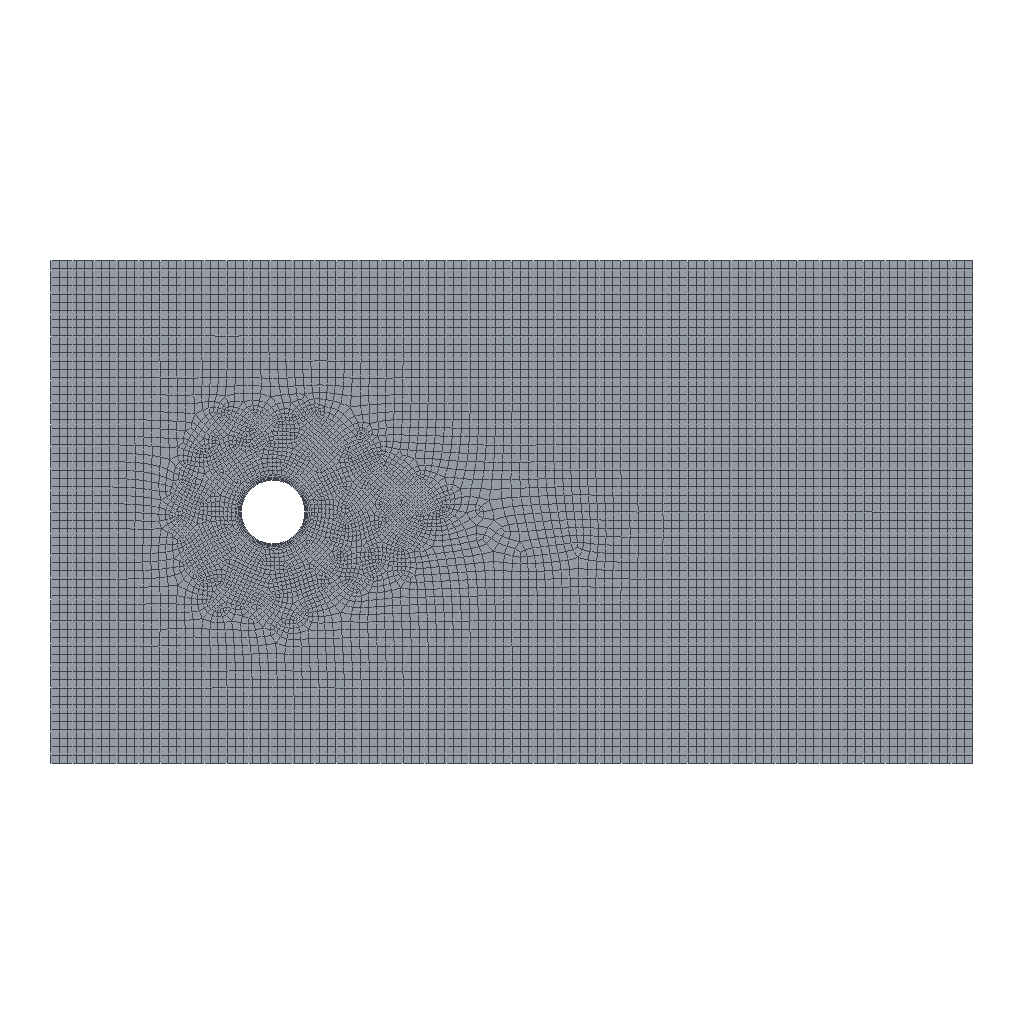Simulation study | ansys fluent
Set-up summary:
category,name,step,type,value,unit,region
solver,ansys_fluent,,Fluent 26.1.0
units,SI m-kg-s (Fluent internal),,stated,boundary values in the units shown in brackets; results in listed units
analysis,deck-1.cas,,"cfd unsteady, 1st-order implicit","dimension=2D; solver=2d, dp, pbns, LES, transient (2d, double precision, pressure-based, large eddy simulation, transient); source_case=2.cas"
model,Space,deck-1.cas,,2D
model,Time,deck-1.cas,,"Unsteady, 1st-Order Implicit"
model,Viscous,deck-1.cas,,Large Eddy Simulation
model,Sub-Grid Scale Model,deck-1.cas,,Smagorinsky-Lilly
model,Heat Transfer,deck-1.cas,,Disabled
model,Acoustics,deck-1.cas,,Ffowcs-Williams and Hawkings
model,Multiphase,deck-1.cas,,Disabled
analysis,deck-2.cas,,"cfd unsteady, 1st-order implicit","dimension=2D; solver=2d, dp, pbns, LES, transient (2d, double precision, pressure-based, large eddy simulation, transient); source_case=4.cas"
model,Space,deck-2.cas,,2D
model,Time,deck-2.cas,,"Unsteady, 1st-Order Implicit"
model,Viscous,deck-2.cas,,Large Eddy Simulation
model,Sub-Grid Scale Model,deck-2.cas,,Smagorinsky-Lilly
model,Heat Transfer,deck-2.cas,,Disabled
model,Multiphase,deck-2.cas,,Disabled
analysis,deck-3.cas,,"cfd unsteady, 1st-order implicit","dimension=2D; solver=2d, dp, pbns, LES, transient (2d, double precision, pressure-based, large eddy simulation, transient); source_case=5.cas.h5"
model,Space,deck-3.cas,,2D
model,Time,deck-3.cas,,"Unsteady, 1st-Order Implicit"
model,Viscous,deck-3.cas,,Large Eddy Simulation
model,Sub-Grid Scale Model,deck-3.cas,,Smagorinsky-Lilly
model,Heat Transfer,deck-3.cas,,Disabled
model,Multiphase,deck-3.cas,,Disabled
analysis,deck-4.cas,,"cfd unsteady, 1st-order implicit","dimension=2D; solver=2d, dp, pbns, LES, transient (2d, double precision, pressure-based, large eddy simulation, transient); source_case=.cas.h5"
model,Space,deck-4.cas,,2D
model,Time,deck-4.cas,,"Unsteady, 1st-Order Implicit"
model,Viscous,deck-4.cas,,Large Eddy Simulation
model,Sub-Grid Scale Model,deck-4.cas,,Smagorinsky-Lilly
model,Heat Transfer,deck-4.cas,,Disabled
model,Acoustics,deck-4.cas,,Ffowcs-Williams and Hawkings
model,Multiphase,deck-4.cas,,Disabled
mesh,deck-1.cas,,nodes,9109
mesh,deck-1.cas,,elements,8909
mesh,deck-1.cas,,faces,18018
mesh,deck-1.cas,,note,elements = cells; counts from the case file zone headers
mesh,deck-2.cas,,nodes,9109
mesh,deck-2.cas,,elements,8909
mesh,deck-2.cas,,faces,18018
mesh,deck-2.cas,,note,elements = cells; counts from the case file zone headers
mesh,deck-3.cas,,nodes,9109
mesh,deck-3.cas,,elements,8909
mesh,deck-3.cas,,faces,18018
mesh,deck-3.cas,,note,elements = cells; counts from the case file zone headers
mesh,deck-4.cas,,nodes,9109
mesh,deck-4.cas,,elements,8909
mesh,deck-4.cas,,faces,18018
mesh,deck-4.cas,,note,elements = cells; counts from the case file zone headers
cell_zone,fluid,deck-1.cas,fluid,material=air,,zone 2
cell_zone,fluid,deck-2.cas,fluid,material=air,,zone 2
cell_zone,fluid,deck-3.cas,fluid,material=air,,zone 2
cell_zone,fluid,deck-4.cas,fluid,material=air,,zone 2
material,air (fluid),,Density,1.225,kg/m^3
material,air (fluid),,Viscosity,1.7894e-05,kg/(m s)
material,aluminum (solid),,Density,2719,kg/m^3
bc,cylinder,deck-1.cas,wall,Wall Motion=Stationary Wall; Shear Boundary Condition=No Slip,,zone 3
bc,symm_bottom,deck-1.cas,symmetry,,,zone 4
bc,symm_top,deck-1.cas,symmetry,,,zone 5
bc,outlet,deck-1.cas,pressure-outlet,,,zone 6
bc,inlet,deck-1.cas,velocity-inlet,Velocity Magnitude [m/s]=69.2,,zone 7
bc,cylinder,deck-2.cas,wall,Wall Motion=Stationary Wall; Shear Boundary Condition=No Slip,,zone 3
bc,symm_bottom,deck-2.cas,symmetry,,,zone 4
bc,symm_top,deck-2.cas,symmetry,,,zone 5
bc,outlet,deck-2.cas,pressure-outlet,,,zone 6
bc,inlet,deck-2.cas,velocity-inlet,Velocity Magnitude [m/s]=69.2,,zone 7
bc,cylinder,deck-3.cas,wall,Wall Motion=Stationary Wall; Shear Boundary Condition=No Slip,,zone 3
bc,symm_bottom,deck-3.cas,symmetry,,,zone 4
bc,symm_top,deck-3.cas,symmetry,,,zone 5
bc,outlet,deck-3.cas,pressure-outlet,,,zone 6
bc,inlet,deck-3.cas,velocity-inlet,Velocity Magnitude [m/s]=69.2,,zone 7
bc,cylinder,deck-4.cas,wall,Wall Motion=Stationary Wall; Shear Boundary Condition=No Slip,,zone 3
bc,symm_bottom,deck-4.cas,symmetry,,,zone 4
bc,symm_top,deck-4.cas,symmetry,,,zone 5
bc,outlet,deck-4.cas,pressure-outlet,,,zone 6
bc,inlet,deck-4.cas,velocity-inlet,Velocity Magnitude [m/s]=69.2,,zone 7
Results summary:
result,mass flow rate cylinder,deck-1.cas,,-0,kg/s
result,mass flow rate inlet,deck-1.cas,,25.431,kg/s
result,mass flow rate outlet,deck-1.cas,,-25.431,kg/s
result,mass flow rate Net,deck-1.cas,,-2.44883e-06,kg/s
result,wall force total cylinder,deck-1.cas,,"(50.306, 33.537, 0)",N
result,wall force pressure cylinder,deck-1.cas,,"(47.546, 33.413, 0)",N
result,wall force viscous cylinder,deck-1.cas,,"(2.76, 0.1238, 0)",N
result,wall force total Net,deck-1.cas,,"(50.306, 33.537, 0)",N
result,wall force pressure Net,deck-1.cas,,"(47.546, 33.413, 0)",N
result,wall force viscous Net,deck-1.cas,,"(2.76, 0.1238, 0)",N
result,mass flow rate cylinder,deck-2.cas,,-0,kg/s
result,mass flow rate inlet,deck-2.cas,,25.431,kg/s
result,mass flow rate outlet,deck-2.cas,,-25.431,kg/s
result,mass flow rate Net,deck-2.cas,,8.69725e-07,kg/s
result,wall force total cylinder,deck-2.cas,,"(45.13, -22.556, 0)",N
result,wall force pressure cylinder,deck-2.cas,,"(42.373, -22.639, 0)",N
result,wall force viscous cylinder,deck-2.cas,,"(2.757, 0.08272, 0)",N
result,wall force total Net,deck-2.cas,,"(45.13, -22.556, 0)",N
result,wall force pressure Net,deck-2.cas,,"(42.373, -22.639, 0)",N
result,wall force viscous Net,deck-2.cas,,"(2.757, 0.08272, 0)",N
result,mass flow rate cylinder,deck-3.cas,,-0,kg/s
result,mass flow rate inlet,deck-3.cas,,25.431,kg/s
result,mass flow rate outlet,deck-3.cas,,-25.431,kg/s
result,mass flow rate Net,deck-3.cas,,8.69725e-07,kg/s
result,wall force total cylinder,deck-3.cas,,"(45.13, -22.556, 0)",N
result,wall force pressure cylinder,deck-3.cas,,"(42.373, -22.639, 0)",N
result,wall force viscous cylinder,deck-3.cas,,"(2.757, 0.08272, 0)",N
result,wall force total Net,deck-3.cas,,"(45.13, -22.556, 0)",N
result,wall force pressure Net,deck-3.cas,,"(42.373, -22.639, 0)",N
result,wall force viscous Net,deck-3.cas,,"(2.757, 0.08272, 0)",N
result,mass flow rate cylinder,deck-4.cas,,-0,kg/s
result,mass flow rate inlet,deck-4.cas,,25.431,kg/s
result,mass flow rate outlet,deck-4.cas,,-25.431,kg/s
result,mass flow rate Net,deck-4.cas,,-2.44883e-06,kg/s
result,wall force total cylinder,deck-4.cas,,"(50.306, 33.537, 0)",N
result,wall force pressure cylinder,deck-4.cas,,"(47.546, 33.413, 0)",N
result,wall force viscous cylinder,deck-4.cas,,"(2.76, 0.1238, 0)",N
result,wall force total Net,deck-4.cas,,"(50.306, 33.537, 0)",N
result,wall force pressure Net,deck-4.cas,,"(47.546, 33.413, 0)",N
result,wall force viscous Net,deck-4.cas,,"(2.76, 0.1238, 0)",N